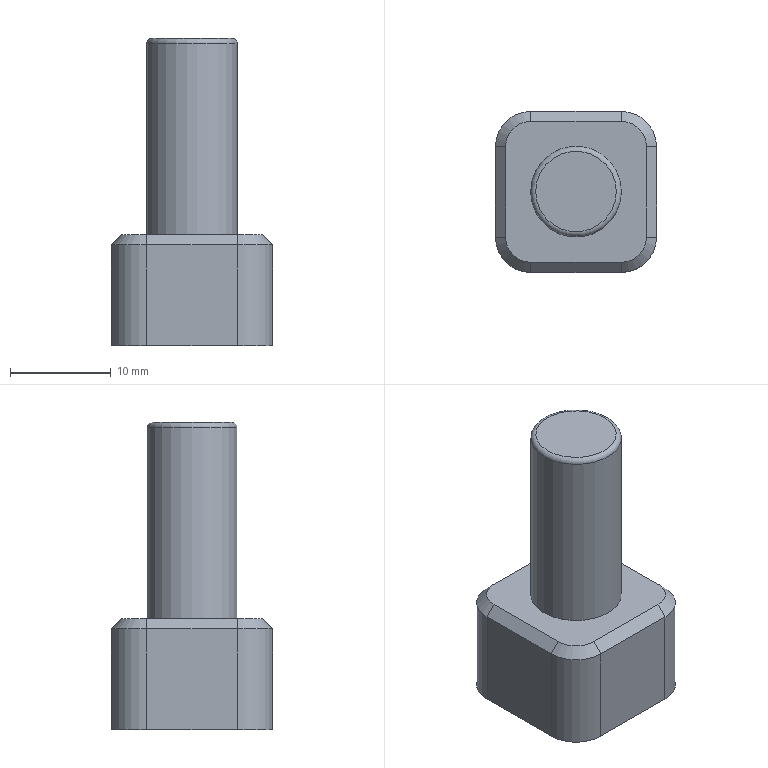NC program | NX | posted with a generic post | part box 16 x 16 x 30.5 mm
Whole program:
N10 G17 G21 G94 G90
(PLANAR_MILL_1 , TOOL : D12-36-D12-75-3T_ROUGH)
N12 T01 M6
N14 G53
N16 G17 G0 G90 X-6.188 Y2.214 S4500 M3
N18 G43 Z51. H1
N20 Z2.
N22 G94 G1 X-6.218 Y2.154 Z1.999 F800.
N24 X-6.55 Y0.628 Z1.972
N26 Y-0.628 Z1.95
N28 X-6.218 Y-2.154 Z1.922
N30 X-5.535 Y-3.558 Z1.895
N32 X-4.54 Y-4.763 Z1.868
N34 X-3.29 Y-5.698 Z1.841
N36 X-1.854 Y-6.313 Z1.813
N38 X-0.314 Y-6.572 Z1.786
N40 X1.244 Y-6.461 Z1.759
N42 X2.731 Y-5.986 Z1.732
N44 X3.819 Y-5.359 Z1.71
N46 X4.87 Y-4.425 Z1.685
N48 X5.698 Y-3.29 Z1.661
N50 X6.267 Y-2.005 Z1.636
N52 X6.55 Y-0.628 Z1.612
N54 Y0.628 Z1.59
N56 X6.267 Y2.005 Z1.565
N58 X5.698 Y3.29 Z1.541
N60 X4.87 Y4.425 Z1.516
N62 X3.819 Y5.359 Z1.491
N64 X2.731 Y5.986 Z1.47
N66 X1.244 Y6.461 Z1.442
N68 X-0.314 Y6.572 Z1.415
N70 X-1.854 Y6.313 Z1.388
N72 X-3.29 Y5.698 Z1.361
N74 X-4.54 Y4.763 Z1.333
N76 X-5.535 Y3.558 Z1.306
N78 X-6.218 Y2.154 Z1.279
N80 X-6.55 Y0.628 Z1.251
N82 Y-0.628 Z1.23
N84 X-6.218 Y-2.154 Z1.202
N86 X-5.535 Y-3.558 Z1.175
N88 X-4.54 Y-4.763 Z1.148
N90 X-3.29 Y-5.698 Z1.121
N92 X-1.854 Y-6.313 Z1.093
N94 X-0.314 Y-6.572 Z1.066
N96 X1.244 Y-6.461 Z1.039
N98 X2.731 Y-5.986 Z1.011
N100 X3.819 Y-5.359 Z0.99
N102 X4.87 Y-4.425 Z0.965
N104 X5.698 Y-3.29 Z0.94
N106 X6.267 Y-2.005 Z0.916
N108 X6.55 Y-0.628 Z0.891
N110 Y0.628 Z0.869
N112 X6.267 Y2.005 Z0.845
N114 X5.698 Y3.29 Z0.82
N116 X4.87 Y4.425 Z0.796
N118 X3.819 Y5.359 Z0.771
N120 X2.731 Y5.986 Z0.749
N122 X1.244 Y6.461 Z0.722
N124 X-0.314 Y6.572 Z0.695
N126 X-1.854 Y6.313 Z0.668
N128 X-3.29 Y5.698 Z0.64
N130 X-4.54 Y4.763 Z0.613
N132 X-5.535 Y3.558 Z0.586
N134 X-6.218 Y2.154 Z0.559
N136 X-6.55 Y0.628 Z0.531
N138 Y-0.628 Z0.509
N140 X-6.218 Y-2.154 Z0.482
N142 X-5.535 Y-3.558 Z0.455
N144 X-4.54 Y-4.763 Z0.428
N146 X-3.29 Y-5.698 Z0.4
N148 X-1.854 Y-6.313 Z0.373
N150 X-0.314 Y-6.572 Z0.346
N152 X1.244 Y-6.461 Z0.319
N154 X2.731 Y-5.986 Z0.291
N156 X3.819 Y-5.359 Z0.269
N158 X4.87 Y-4.425 Z0.245
N160 X5.698 Y-3.29 Z0.22
N162 X6.267 Y-2.005 Z0.196
N164 X6.55 Y-0.628 Z0.171
N166 Y0.628 Z0.149
N168 X6.267 Y2.005 Z0.125
N170 X5.698 Y3.29 Z0.1
N172 X4.87 Y4.425 Z0.076
N174 X3.819 Y5.359 Z0.051
N176 X2.731 Y5.986 Z0.029
N178 X1.244 Y6.461 Z0.002
N180 X-0.314 Y6.572 Z-0.025
N182 X-1.854 Y6.313 Z-0.052
N184 X-3.29 Y5.698 Z-0.08
N186 X-4.54 Y4.763 Z-0.107
N188 X-5.535 Y3.558 Z-0.134
N190 X-6.218 Y2.154 Z-0.162
N192 X-6.55 Y0.628 Z-0.189
N194 Y-0.628 Z-0.211
N196 X-6.218 Y-2.154 Z-0.238
N198 X-5.535 Y-3.558 Z-0.265
N200 X-4.54 Y-4.763 Z-0.292
N202 X-3.29 Y-5.698 Z-0.32
N204 X-1.854 Y-6.313 Z-0.347
N206 X-0.314 Y-6.572 Z-0.374
N208 X1.244 Y-6.461 Z-0.402
N210 X2.731 Y-5.986 Z-0.429
N212 X3.819 Y-5.359 Z-0.451
N214 X4.87 Y-4.425 Z-0.475
N216 X5.698 Y-3.29 Z-0.5
N218 X6.267 Y-2.005 Z-0.524
N220 X6.55 Y-0.628 Z-0.549
N222 Y0.628 Z-0.571
N224 X6.267 Y2.005 Z-0.595
N226 X5.698 Y3.29 Z-0.62
N228 X4.87 Y4.425 Z-0.644
N230 X3.819 Y5.359 Z-0.669
N232 X2.731 Y5.986 Z-0.691
N234 X1.244 Y6.461 Z-0.718
N236 X-0.314 Y6.572 Z-0.745
N238 X-1.854 Y6.313 Z-0.773
N240 X-3.29 Y5.698 Z-0.8
N242 X-4.54 Y4.763 Z-0.827
N244 X-5.535 Y3.558 Z-0.854
N246 X-6.218 Y2.154 Z-0.882
N248 X-6.55 Y0.628 Z-0.909
N250 Y-0.628 Z-0.931
N252 X-6.218 Y-2.154 Z-0.958
N254 X-5.535 Y-3.558 Z-0.985
N256 X-4.54 Y-4.763 Z-1.013
N258 X-3.29 Y-5.698 Z-1.04
N260 X-1.854 Y-6.313 Z-1.067
N262 X-0.314 Y-6.572 Z-1.094
N264 X1.244 Y-6.461 Z-1.122
N266 X2.731 Y-5.986 Z-1.149
N268 X3.819 Y-5.359 Z-1.171
N270 X4.87 Y-4.425 Z-1.195
N272 X5.698 Y-3.29 Z-1.22
N274 X6.267 Y-2.005 Z-1.244
N276 X6.55 Y-0.628 Z-1.269
N278 Y0.628 Z-1.291
N280 X6.267 Y2.005 Z-1.315
N282 X5.698 Y3.29 Z-1.34
N284 X4.87 Y4.425 Z-1.364
N286 X3.819 Y5.359 Z-1.389
N288 X2.731 Y5.986 Z-1.411
N290 X1.244 Y6.461 Z-1.438
N292 X-0.314 Y6.572 Z-1.465
N294 X-1.854 Y6.313 Z-1.493
N296 X-3.29 Y5.698 Z-1.52
N298 X-4.54 Y4.763 Z-1.547
N300 X-5.535 Y3.558 Z-1.574
N302 X-6.218 Y2.154 Z-1.602
N304 X-6.55 Y0.628 Z-1.629
N306 Y-0.628 Z-1.651
N308 X-6.218 Y-2.154 Z-1.678
N310 X-5.535 Y-3.558 Z-1.705
N312 X-4.54 Y-4.763 Z-1.733
N314 X-3.29 Y-5.698 Z-1.76
N316 X-1.854 Y-6.313 Z-1.787
N318 X-0.314 Y-6.572 Z-1.814
N320 X1.244 Y-6.461 Z-1.842
N322 X2.731 Y-5.986 Z-1.869
N324 X3.819 Y-5.359 Z-1.891
N326 X4.87 Y-4.425 Z-1.915
N328 X5.698 Y-3.29 Z-1.94
N330 X6.267 Y-2.005 Z-1.965
N332 X6.55 Y-0.628 Z-1.989
N334 Y0. Z-2.
N336 G3 X0. Y6.55 R6.55
N338 X6.55 Y0. R-6.55
N340 G1 Z-1.
N342 G0 Z51.
N344 M5
N346 M2